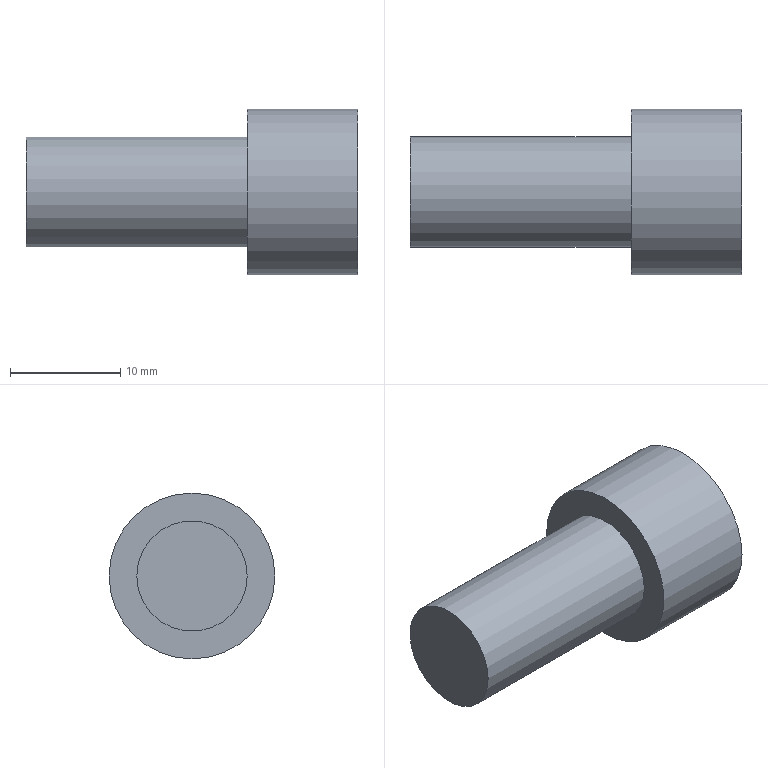Part | NX | features solid 2 | 1 solid | 12 faces | box 30 x 15 x 15 mm | volume 3005 mm3 | plane 10 | cylinder 2 | commonest cylinder face diameters 10 x1 15 x1
STEP:
#1=CARTESIAN_POINT('',(1054.,-177.,-457.691));
#2=VERTEX_POINT('',#1);
#3=CARTESIAN_POINT('',(1054.,-181.,-455.381));
#4=VERTEX_POINT('',#3);
#5=CARTESIAN_POINT('',(1054.,-179.,-456.536));
#6=DIRECTION('',(0.,-0.866,0.5));
#7=VECTOR('',#6,1000.);
#8=LINE('',#5,#7);
#9=EDGE_CURVE('',#2,#4,#8,.T.);
#10=ORIENTED_EDGE('',*,*,#9,.F.);
#11=CARTESIAN_POINT('',(1054.,-177.,-462.309));
#12=VERTEX_POINT('',#11);
#13=CARTESIAN_POINT('',(1054.,-177.,-460.));
#14=DIRECTION('',(0.,0.,1.));
#15=VECTOR('',#14,1000.);
#16=LINE('',#13,#15);
#17=EDGE_CURVE('',#12,#2,#16,.T.);
#18=ORIENTED_EDGE('',*,*,#17,.F.);
#19=CARTESIAN_POINT('',(1054.,-181.,-464.619));
#20=VERTEX_POINT('',#19);
#21=CARTESIAN_POINT('',(1054.,-179.,-463.464));
#22=DIRECTION('',(0.,0.866,0.5));
#23=VECTOR('',#22,1000.);
#24=LINE('',#21,#23);
#25=EDGE_CURVE('',#20,#12,#24,.T.);
#26=ORIENTED_EDGE('',*,*,#25,.F.);
#27=CARTESIAN_POINT('',(1054.,-185.,-462.309));
#28=VERTEX_POINT('',#27);
#29=CARTESIAN_POINT('',(1054.,-183.,-463.464));
#30=DIRECTION('',(0.,0.866,-0.5));
#31=VECTOR('',#30,1000.);
#32=LINE('',#29,#31);
#33=EDGE_CURVE('',#28,#20,#32,.T.);
#34=ORIENTED_EDGE('',*,*,#33,.F.);
#35=CARTESIAN_POINT('',(1054.,-185.,-457.691));
#36=VERTEX_POINT('',#35);
#37=CARTESIAN_POINT('',(1054.,-185.,-460.));
#38=DIRECTION('',(0.,0.,-1.));
#39=VECTOR('',#38,1000.);
#40=LINE('',#37,#39);
#41=EDGE_CURVE('',#36,#28,#40,.T.);
#42=ORIENTED_EDGE('',*,*,#41,.F.);
#43=CARTESIAN_POINT('',(1054.,-183.,-456.536));
#44=DIRECTION('',(0.,-0.866,-0.5));
#45=VECTOR('',#44,1000.);
#46=LINE('',#43,#45);
#47=EDGE_CURVE('',#4,#36,#46,.T.);
#48=ORIENTED_EDGE('',*,*,#47,.F.);
#49=EDGE_LOOP('',(#10,#18,#26,#34,#42,#48));
#50=FACE_BOUND('',#49,.T.);
#51=CARTESIAN_POINT('',(1054.,-173.5,-460.));
#52=VERTEX_POINT('',#51);
#53=CARTESIAN_POINT('',(1054.,-181.,-460.));
#54=DIRECTION('',(-1.,0.,0.));
#55=DIRECTION('',(0.,1.,0.));
#56=AXIS2_PLACEMENT_3D('',#53,#54,#55);
#57=CIRCLE('',#56,7.5);
#58=EDGE_CURVE('',#52,#52,#57,.T.);
#59=ORIENTED_EDGE('',*,*,#58,.F.);
#60=EDGE_LOOP('',(#59));
#61=FACE_BOUND('',#60,.T.);
#62=CARTESIAN_POINT('',(1054.,-181.,-460.));
#63=DIRECTION('',(1.,0.,0.));
#64=DIRECTION('',(0.,-1.,0.));
#65=AXIS2_PLACEMENT_3D('',#62,#63,#64);
#66=PLANE('',#65);
#67=ADVANCED_FACE('',(#50,#61),#66,.T.);
#68=CARTESIAN_POINT('',(1044.,-176.,-460.));
#69=VERTEX_POINT('',#68);
#70=CARTESIAN_POINT('',(1044.,-181.,-460.));
#71=DIRECTION('',(-1.,0.,0.));
#72=DIRECTION('',(0.,1.,0.));
#73=AXIS2_PLACEMENT_3D('',#70,#71,#72);
#74=CIRCLE('',#73,5.);
#75=EDGE_CURVE('',#69,#69,#74,.T.);
#76=ORIENTED_EDGE('',*,*,#75,.F.);
#77=EDGE_LOOP('',(#76));
#78=FACE_BOUND('',#77,.T.);
#79=CARTESIAN_POINT('',(1044.,-188.5,-460.));
#80=VERTEX_POINT('',#79);
#81=CARTESIAN_POINT('',(1044.,-181.,-460.));
#82=DIRECTION('',(1.,0.,0.));
#83=DIRECTION('',(0.,-1.,0.));
#84=AXIS2_PLACEMENT_3D('',#81,#82,#83);
#85=CIRCLE('',#84,7.5);
#86=EDGE_CURVE('',#80,#80,#85,.T.);
#87=ORIENTED_EDGE('',*,*,#86,.F.);
#88=EDGE_LOOP('',(#87));
#89=FACE_BOUND('',#88,.T.);
#90=CARTESIAN_POINT('',(1044.,-181.,-460.));
#91=DIRECTION('',(-1.,0.,0.));
#92=DIRECTION('',(0.,1.,0.));
#93=AXIS2_PLACEMENT_3D('',#90,#91,#92);
#94=PLANE('',#93);
#95=ADVANCED_FACE('',(#78,#89),#94,.T.);
#96=ORIENTED_EDGE('',*,*,#58,.T.);
#97=EDGE_LOOP('',(#96));
#98=FACE_BOUND('',#97,.T.);
#99=ORIENTED_EDGE('',*,*,#86,.T.);
#100=EDGE_LOOP('',(#99));
#101=FACE_BOUND('',#100,.T.);
#102=CARTESIAN_POINT('',(1044.,-181.,-460.));
#103=DIRECTION('',(1.,0.,0.));
#104=DIRECTION('',(0.,-1.,0.));
#105=AXIS2_PLACEMENT_3D('',#102,#103,#104);
#106=CYLINDRICAL_SURFACE('',#105,7.5);
#107=ADVANCED_FACE('',(#98,#101),#106,.T.);
#108=ORIENTED_EDGE('',*,*,#9,.T.);
#109=CARTESIAN_POINT('',(1048.,-181.,-455.381));
#110=VERTEX_POINT('',#109);
#111=CARTESIAN_POINT('',(1048.,-181.,-455.381));
#112=DIRECTION('',(1.,0.,0.));
#113=VECTOR('',#112,1000.);
#114=LINE('',#111,#113);
#115=EDGE_CURVE('',#110,#4,#114,.T.);
#116=ORIENTED_EDGE('',*,*,#115,.F.);
#117=CARTESIAN_POINT('',(1048.,-177.,-457.691));
#118=VERTEX_POINT('',#117);
#119=CARTESIAN_POINT('',(1048.,-177.,-457.691));
#120=DIRECTION('',(0.,-0.866,0.5));
#121=VECTOR('',#120,1000.);
#122=LINE('',#119,#121);
#123=EDGE_CURVE('',#118,#110,#122,.T.);
#124=ORIENTED_EDGE('',*,*,#123,.F.);
#125=CARTESIAN_POINT('',(1048.,-177.,-457.691));
#126=DIRECTION('',(1.,0.,0.));
#127=VECTOR('',#126,1000.);
#128=LINE('',#125,#127);
#129=EDGE_CURVE('',#118,#2,#128,.T.);
#130=ORIENTED_EDGE('',*,*,#129,.T.);
#131=EDGE_LOOP('',(#108,#116,#124,#130));
#132=FACE_BOUND('',#131,.T.);
#133=CARTESIAN_POINT('',(1053.,-179.,-456.536));
#134=DIRECTION('',(0.,0.5,0.866));
#135=DIRECTION('',(0.,-0.866,0.5));
#136=AXIS2_PLACEMENT_3D('',#133,#134,#135);
#137=PLANE('',#136);
#138=ADVANCED_FACE('',(#132),#137,.F.);
#139=ORIENTED_EDGE('',*,*,#17,.T.);
#140=ORIENTED_EDGE('',*,*,#129,.F.);
#141=CARTESIAN_POINT('',(1048.,-177.,-462.309));
#142=VERTEX_POINT('',#141);
#143=CARTESIAN_POINT('',(1048.,-177.,-462.309));
#144=DIRECTION('',(0.,0.,1.));
#145=VECTOR('',#144,1000.);
#146=LINE('',#143,#145);
#147=EDGE_CURVE('',#142,#118,#146,.T.);
#148=ORIENTED_EDGE('',*,*,#147,.F.);
#149=CARTESIAN_POINT('',(1048.,-177.,-462.309));
#150=DIRECTION('',(1.,0.,0.));
#151=VECTOR('',#150,1000.);
#152=LINE('',#149,#151);
#153=EDGE_CURVE('',#142,#12,#152,.T.);
#154=ORIENTED_EDGE('',*,*,#153,.T.);
#155=EDGE_LOOP('',(#139,#140,#148,#154));
#156=FACE_BOUND('',#155,.T.);
#157=CARTESIAN_POINT('',(1053.,-177.,-460.));
#158=DIRECTION('',(0.,1.,0.));
#159=DIRECTION('',(0.,0.,1.));
#160=AXIS2_PLACEMENT_3D('',#157,#158,#159);
#161=PLANE('',#160);
#162=ADVANCED_FACE('',(#156),#161,.F.);
#163=ORIENTED_EDGE('',*,*,#25,.T.);
#164=ORIENTED_EDGE('',*,*,#153,.F.);
#165=CARTESIAN_POINT('',(1048.,-181.,-464.619));
#166=VERTEX_POINT('',#165);
#167=CARTESIAN_POINT('',(1048.,-181.,-464.619));
#168=DIRECTION('',(0.,0.866,0.5));
#169=VECTOR('',#168,1000.);
#170=LINE('',#167,#169);
#171=EDGE_CURVE('',#166,#142,#170,.T.);
#172=ORIENTED_EDGE('',*,*,#171,.F.);
#173=CARTESIAN_POINT('',(1048.,-181.,-464.619));
#174=DIRECTION('',(1.,0.,0.));
#175=VECTOR('',#174,1000.);
#176=LINE('',#173,#175);
#177=EDGE_CURVE('',#166,#20,#176,.T.);
#178=ORIENTED_EDGE('',*,*,#177,.T.);
#179=EDGE_LOOP('',(#163,#164,#172,#178));
#180=FACE_BOUND('',#179,.T.);
#181=CARTESIAN_POINT('',(1053.,-179.,-463.464));
#182=DIRECTION('',(0.,0.5,-0.866));
#183=DIRECTION('',(0.,0.866,0.5));
#184=AXIS2_PLACEMENT_3D('',#181,#182,#183);
#185=PLANE('',#184);
#186=ADVANCED_FACE('',(#180),#185,.F.);
#187=ORIENTED_EDGE('',*,*,#33,.T.);
#188=ORIENTED_EDGE('',*,*,#177,.F.);
#189=CARTESIAN_POINT('',(1048.,-185.,-462.309));
#190=VERTEX_POINT('',#189);
#191=CARTESIAN_POINT('',(1048.,-185.,-462.309));
#192=DIRECTION('',(0.,0.866,-0.5));
#193=VECTOR('',#192,1000.);
#194=LINE('',#191,#193);
#195=EDGE_CURVE('',#190,#166,#194,.T.);
#196=ORIENTED_EDGE('',*,*,#195,.F.);
#197=CARTESIAN_POINT('',(1048.,-185.,-462.309));
#198=DIRECTION('',(1.,0.,0.));
#199=VECTOR('',#198,1000.);
#200=LINE('',#197,#199);
#201=EDGE_CURVE('',#190,#28,#200,.T.);
#202=ORIENTED_EDGE('',*,*,#201,.T.);
#203=EDGE_LOOP('',(#187,#188,#196,#202));
#204=FACE_BOUND('',#203,.T.);
#205=CARTESIAN_POINT('',(1053.,-183.,-463.464));
#206=DIRECTION('',(0.,-0.5,-0.866));
#207=DIRECTION('',(0.,0.866,-0.5));
#208=AXIS2_PLACEMENT_3D('',#205,#206,#207);
#209=PLANE('',#208);
#210=ADVANCED_FACE('',(#204),#209,.F.);
#211=ORIENTED_EDGE('',*,*,#41,.T.);
#212=ORIENTED_EDGE('',*,*,#201,.F.);
#213=CARTESIAN_POINT('',(1048.,-185.,-457.691));
#214=VERTEX_POINT('',#213);
#215=CARTESIAN_POINT('',(1048.,-185.,-457.691));
#216=DIRECTION('',(0.,0.,-1.));
#217=VECTOR('',#216,1000.);
#218=LINE('',#215,#217);
#219=EDGE_CURVE('',#214,#190,#218,.T.);
#220=ORIENTED_EDGE('',*,*,#219,.F.);
#221=CARTESIAN_POINT('',(1048.,-185.,-457.691));
#222=DIRECTION('',(1.,0.,0.));
#223=VECTOR('',#222,1000.);
#224=LINE('',#221,#223);
#225=EDGE_CURVE('',#214,#36,#224,.T.);
#226=ORIENTED_EDGE('',*,*,#225,.T.);
#227=EDGE_LOOP('',(#211,#212,#220,#226));
#228=FACE_BOUND('',#227,.T.);
#229=CARTESIAN_POINT('',(1053.,-185.,-460.));
#230=DIRECTION('',(0.,-1.,0.));
#231=DIRECTION('',(0.,0.,-1.));
#232=AXIS2_PLACEMENT_3D('',#229,#230,#231);
#233=PLANE('',#232);
#234=ADVANCED_FACE('',(#228),#233,.F.);
#235=ORIENTED_EDGE('',*,*,#47,.T.);
#236=ORIENTED_EDGE('',*,*,#225,.F.);
#237=CARTESIAN_POINT('',(1048.,-181.,-455.381));
#238=DIRECTION('',(0.,-0.866,-0.5));
#239=VECTOR('',#238,1000.);
#240=LINE('',#237,#239);
#241=EDGE_CURVE('',#110,#214,#240,.T.);
#242=ORIENTED_EDGE('',*,*,#241,.F.);
#243=ORIENTED_EDGE('',*,*,#115,.T.);
#244=EDGE_LOOP('',(#235,#236,#242,#243));
#245=FACE_BOUND('',#244,.T.);
#246=CARTESIAN_POINT('',(1053.,-183.,-456.536));
#247=DIRECTION('',(0.,-0.5,0.866));
#248=DIRECTION('',(0.,-0.866,-0.5));
#249=AXIS2_PLACEMENT_3D('',#246,#247,#248);
#250=PLANE('',#249);
#251=ADVANCED_FACE('',(#245),#250,.F.);
#252=ORIENTED_EDGE('',*,*,#241,.T.);
#253=ORIENTED_EDGE('',*,*,#219,.T.);
#254=ORIENTED_EDGE('',*,*,#195,.T.);
#255=ORIENTED_EDGE('',*,*,#171,.T.);
#256=ORIENTED_EDGE('',*,*,#147,.T.);
#257=ORIENTED_EDGE('',*,*,#123,.T.);
#258=EDGE_LOOP('',(#252,#253,#254,#255,#256,#257));
#259=FACE_BOUND('',#258,.T.);
#260=CARTESIAN_POINT('',(1048.,-181.,-460.));
#261=DIRECTION('',(-1.,0.,0.));
#262=DIRECTION('',(0.,1.,0.));
#263=AXIS2_PLACEMENT_3D('',#260,#261,#262);
#264=PLANE('',#263);
#265=ADVANCED_FACE('',(#259),#264,.F.);
#266=CARTESIAN_POINT('',(1024.,-186.,-460.));
#267=VERTEX_POINT('',#266);
#268=CARTESIAN_POINT('',(1024.,-181.,-460.));
#269=DIRECTION('',(1.,0.,0.));
#270=DIRECTION('',(0.,-1.,0.));
#271=AXIS2_PLACEMENT_3D('',#268,#269,#270);
#272=CIRCLE('',#271,5.);
#273=EDGE_CURVE('',#267,#267,#272,.T.);
#274=ORIENTED_EDGE('',*,*,#273,.F.);
#275=EDGE_LOOP('',(#274));
#276=FACE_BOUND('',#275,.T.);
#277=CARTESIAN_POINT('',(1024.,-181.,-460.));
#278=DIRECTION('',(-1.,0.,0.));
#279=DIRECTION('',(0.,1.,0.));
#280=AXIS2_PLACEMENT_3D('',#277,#278,#279);
#281=PLANE('',#280);
#282=ADVANCED_FACE('',(#276),#281,.T.);
#283=ORIENTED_EDGE('',*,*,#273,.T.);
#284=EDGE_LOOP('',(#283));
#285=FACE_BOUND('',#284,.T.);
#286=ORIENTED_EDGE('',*,*,#75,.T.);
#287=EDGE_LOOP('',(#286));
#288=FACE_BOUND('',#287,.T.);
#289=CARTESIAN_POINT('',(1044.,-181.,-460.));
#290=DIRECTION('',(-1.,0.,0.));
#291=DIRECTION('',(0.,1.,0.));
#292=AXIS2_PLACEMENT_3D('',#289,#290,#291);
#293=CYLINDRICAL_SURFACE('',#292,5.);
#294=ADVANCED_FACE('',(#285,#288),#293,.T.);
#295=CLOSED_SHELL('',(#67,#95,#107,#138,#162,#186,#210,#234,#251,#265,#282,#294));
#296=MANIFOLD_SOLID_BREP('',#295);
#297=(LENGTH_UNIT()NAMED_UNIT(*)SI_UNIT(.MILLI.,.METRE.));
#298=UNCERTAINTY_MEASURE_WITH_UNIT(LENGTH_MEASURE(0.00001),#297,'','');
#299=(NAMED_UNIT(*)PLANE_ANGLE_UNIT()SI_UNIT($,.RADIAN.));
#300=(NAMED_UNIT(*)SI_UNIT($,.STERADIAN.)SOLID_ANGLE_UNIT());
#301=(GEOMETRIC_REPRESENTATION_CONTEXT(3)GLOBAL_UNCERTAINTY_ASSIGNED_CONTEXT((#298))GLOBAL_UNIT_ASSIGNED_CONTEXT((#297,#299,#300))REPRESENTATION_CONTEXT('',''));
#302=ADVANCED_BREP_SHAPE_REPRESENTATION('',(#296),#301);